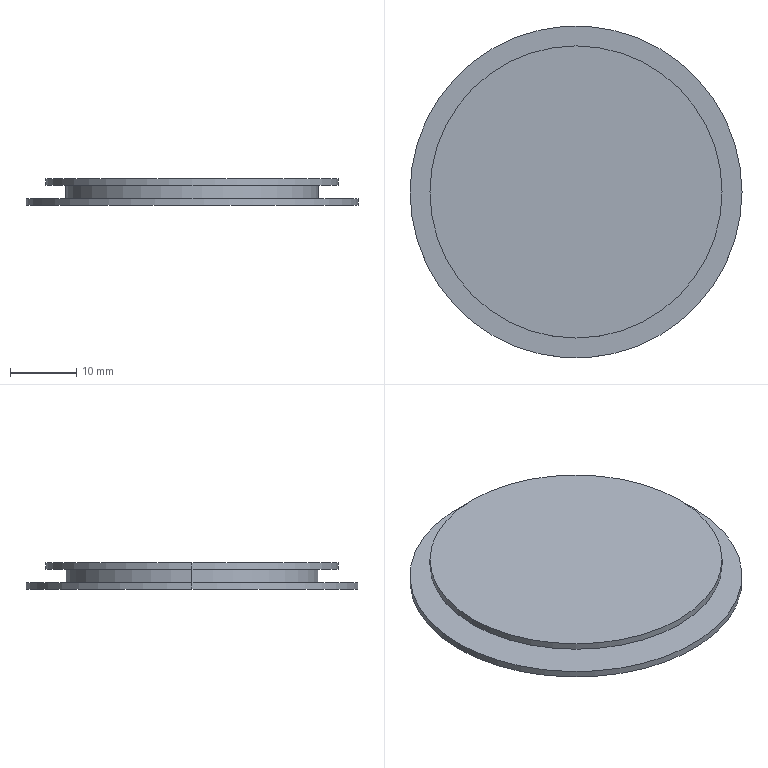Part | SolidWorks | features ICE 2, Extrusion 1 | 1 solid | 10 faces | box 50 x 50 x 4 mm | volume 5752 mm3 | cylinder 6 | plane 4 | commonest cylinder face diameters 38 x2 44 x2 50 x2
STEP:
#1=CARTESIAN_POINT('',(22.,0.,4.));
#2=VERTEX_POINT('',#1);
#3=CARTESIAN_POINT('',(-22.,0.,4.));
#4=VERTEX_POINT('',#3);
#5=CARTESIAN_POINT('',(0.,0.,4.));
#6=DIRECTION('',(0.,0.,1.));
#7=DIRECTION('',(1.,0.,0.));
#8=AXIS2_PLACEMENT_3D('',#5,#6,#7);
#9=CIRCLE('',#8,22.);
#10=EDGE_CURVE('',#2,#4,#9,.T.);
#11=ORIENTED_EDGE('',*,*,#10,.F.);
#12=CARTESIAN_POINT('',(22.,0.,3.));
#13=VERTEX_POINT('',#12);
#14=CARTESIAN_POINT('',(22.,0.,4.));
#15=DIRECTION('',(0.,0.,-1.));
#16=VECTOR('',#15,1000.);
#17=LINE('',#14,#16);
#18=EDGE_CURVE('',#2,#13,#17,.T.);
#19=ORIENTED_EDGE('',*,*,#18,.T.);
#20=CARTESIAN_POINT('',(-22.,0.,3.));
#21=VERTEX_POINT('',#20);
#22=CARTESIAN_POINT('',(0.,0.,3.));
#23=DIRECTION('',(0.,0.,1.));
#24=DIRECTION('',(1.,0.,0.));
#25=AXIS2_PLACEMENT_3D('',#22,#23,#24);
#26=CIRCLE('',#25,22.);
#27=EDGE_CURVE('',#13,#21,#26,.T.);
#28=ORIENTED_EDGE('',*,*,#27,.T.);
#29=CARTESIAN_POINT('',(-22.,0.,4.));
#30=DIRECTION('',(0.,0.,-1.));
#31=VECTOR('',#30,1000.);
#32=LINE('',#29,#31);
#33=EDGE_CURVE('',#4,#21,#32,.T.);
#34=ORIENTED_EDGE('',*,*,#33,.F.);
#35=EDGE_LOOP('',(#11,#19,#28,#34));
#36=FACE_OUTER_BOUND('',#35,.T.);
#37=CARTESIAN_POINT('',(0.,0.,4.));
#38=DIRECTION('',(0.,0.,-1.));
#39=DIRECTION('',(-1.,0.,0.));
#40=AXIS2_PLACEMENT_3D('',#37,#38,#39);
#41=CYLINDRICAL_SURFACE('',#40,22.);
#42=ADVANCED_FACE('',(#36),#41,.T.);
#43=CARTESIAN_POINT('',(19.,0.,3.));
#44=VERTEX_POINT('',#43);
#45=CARTESIAN_POINT('',(-19.,0.,3.));
#46=VERTEX_POINT('',#45);
#47=CARTESIAN_POINT('',(0.,0.,3.));
#48=DIRECTION('',(0.,0.,1.));
#49=DIRECTION('',(1.,0.,0.));
#50=AXIS2_PLACEMENT_3D('',#47,#48,#49);
#51=CIRCLE('',#50,19.);
#52=EDGE_CURVE('',#44,#46,#51,.T.);
#53=ORIENTED_EDGE('',*,*,#52,.F.);
#54=CARTESIAN_POINT('',(19.,0.,1.));
#55=VERTEX_POINT('',#54);
#56=CARTESIAN_POINT('',(19.,0.,3.));
#57=DIRECTION('',(0.,0.,-1.));
#58=VECTOR('',#57,1000.);
#59=LINE('',#56,#58);
#60=EDGE_CURVE('',#44,#55,#59,.T.);
#61=ORIENTED_EDGE('',*,*,#60,.T.);
#62=CARTESIAN_POINT('',(-19.,0.,1.));
#63=VERTEX_POINT('',#62);
#64=CARTESIAN_POINT('',(0.,0.,1.));
#65=DIRECTION('',(0.,0.,1.));
#66=DIRECTION('',(1.,0.,0.));
#67=AXIS2_PLACEMENT_3D('',#64,#65,#66);
#68=CIRCLE('',#67,19.);
#69=EDGE_CURVE('',#55,#63,#68,.T.);
#70=ORIENTED_EDGE('',*,*,#69,.T.);
#71=CARTESIAN_POINT('',(-19.,0.,3.));
#72=DIRECTION('',(0.,0.,-1.));
#73=VECTOR('',#72,1000.);
#74=LINE('',#71,#73);
#75=EDGE_CURVE('',#46,#63,#74,.T.);
#76=ORIENTED_EDGE('',*,*,#75,.F.);
#77=EDGE_LOOP('',(#53,#61,#70,#76));
#78=FACE_OUTER_BOUND('',#77,.T.);
#79=CARTESIAN_POINT('',(0.,0.,3.));
#80=DIRECTION('',(0.,0.,-1.));
#81=DIRECTION('',(-1.,0.,0.));
#82=AXIS2_PLACEMENT_3D('',#79,#80,#81);
#83=CYLINDRICAL_SURFACE('',#82,19.);
#84=ADVANCED_FACE('',(#78),#83,.T.);
#85=CARTESIAN_POINT('',(25.,0.,1.));
#86=VERTEX_POINT('',#85);
#87=CARTESIAN_POINT('',(-25.,0.,1.));
#88=VERTEX_POINT('',#87);
#89=CARTESIAN_POINT('',(0.,0.,1.));
#90=DIRECTION('',(0.,0.,1.));
#91=DIRECTION('',(1.,0.,0.));
#92=AXIS2_PLACEMENT_3D('',#89,#90,#91);
#93=CIRCLE('',#92,25.);
#94=EDGE_CURVE('',#86,#88,#93,.T.);
#95=ORIENTED_EDGE('',*,*,#94,.F.);
#96=CARTESIAN_POINT('',(25.,0.,0.));
#97=VERTEX_POINT('',#96);
#98=CARTESIAN_POINT('',(25.,0.,1.));
#99=DIRECTION('',(0.,0.,-1.));
#100=VECTOR('',#99,1000.);
#101=LINE('',#98,#100);
#102=EDGE_CURVE('',#86,#97,#101,.T.);
#103=ORIENTED_EDGE('',*,*,#102,.T.);
#104=CARTESIAN_POINT('',(-25.,0.,0.));
#105=VERTEX_POINT('',#104);
#106=CARTESIAN_POINT('',(0.,0.,0.));
#107=DIRECTION('',(0.,0.,1.));
#108=DIRECTION('',(1.,0.,0.));
#109=AXIS2_PLACEMENT_3D('',#106,#107,#108);
#110=CIRCLE('',#109,25.);
#111=EDGE_CURVE('',#97,#105,#110,.T.);
#112=ORIENTED_EDGE('',*,*,#111,.T.);
#113=CARTESIAN_POINT('',(-25.,0.,1.));
#114=DIRECTION('',(0.,0.,-1.));
#115=VECTOR('',#114,1000.);
#116=LINE('',#113,#115);
#117=EDGE_CURVE('',#88,#105,#116,.T.);
#118=ORIENTED_EDGE('',*,*,#117,.F.);
#119=EDGE_LOOP('',(#95,#103,#112,#118));
#120=FACE_OUTER_BOUND('',#119,.T.);
#121=CARTESIAN_POINT('',(0.,0.,1.));
#122=DIRECTION('',(0.,0.,-1.));
#123=DIRECTION('',(-1.,0.,0.));
#124=AXIS2_PLACEMENT_3D('',#121,#122,#123);
#125=CYLINDRICAL_SURFACE('',#124,25.);
#126=ADVANCED_FACE('',(#120),#125,.T.);
#127=ORIENTED_EDGE('',*,*,#102,.F.);
#128=CARTESIAN_POINT('',(0.,0.,1.));
#129=DIRECTION('',(0.,0.,1.));
#130=DIRECTION('',(1.,0.,0.));
#131=AXIS2_PLACEMENT_3D('',#128,#129,#130);
#132=CIRCLE('',#131,25.);
#133=EDGE_CURVE('',#88,#86,#132,.T.);
#134=ORIENTED_EDGE('',*,*,#133,.F.);
#135=ORIENTED_EDGE('',*,*,#117,.T.);
#136=CARTESIAN_POINT('',(0.,0.,0.));
#137=DIRECTION('',(0.,0.,1.));
#138=DIRECTION('',(1.,0.,0.));
#139=AXIS2_PLACEMENT_3D('',#136,#137,#138);
#140=CIRCLE('',#139,25.);
#141=EDGE_CURVE('',#105,#97,#140,.T.);
#142=ORIENTED_EDGE('',*,*,#141,.T.);
#143=EDGE_LOOP('',(#127,#134,#135,#142));
#144=FACE_OUTER_BOUND('',#143,.T.);
#145=CARTESIAN_POINT('',(0.,0.,1.));
#146=DIRECTION('',(0.,0.,-1.));
#147=DIRECTION('',(-1.,0.,0.));
#148=AXIS2_PLACEMENT_3D('',#145,#146,#147);
#149=CYLINDRICAL_SURFACE('',#148,25.);
#150=ADVANCED_FACE('',(#144),#149,.T.);
#151=CARTESIAN_POINT('',(0.,0.,1.));
#152=DIRECTION('',(0.,0.,1.));
#153=DIRECTION('',(1.,0.,0.));
#154=AXIS2_PLACEMENT_3D('',#151,#152,#153);
#155=CIRCLE('',#154,19.);
#156=EDGE_CURVE('',#63,#55,#155,.T.);
#157=ORIENTED_EDGE('',*,*,#156,.F.);
#158=ORIENTED_EDGE('',*,*,#69,.F.);
#159=EDGE_LOOP('',(#157,#158));
#160=FACE_BOUND('',#159,.T.);
#161=ORIENTED_EDGE('',*,*,#133,.T.);
#162=ORIENTED_EDGE('',*,*,#94,.T.);
#163=EDGE_LOOP('',(#161,#162));
#164=FACE_OUTER_BOUND('',#163,.T.);
#165=CARTESIAN_POINT('',(0.,0.,1.));
#166=DIRECTION('',(0.,0.,1.));
#167=DIRECTION('',(1.,0.,0.));
#168=AXIS2_PLACEMENT_3D('',#165,#166,#167);
#169=PLANE('',#168);
#170=ADVANCED_FACE('',(#160,#164),#169,.T.);
#171=ORIENTED_EDGE('',*,*,#141,.F.);
#172=ORIENTED_EDGE('',*,*,#111,.F.);
#173=EDGE_LOOP('',(#171,#172));
#174=FACE_OUTER_BOUND('',#173,.T.);
#175=CARTESIAN_POINT('',(0.,0.,0.));
#176=DIRECTION('',(0.,0.,1.));
#177=DIRECTION('',(1.,0.,0.));
#178=AXIS2_PLACEMENT_3D('',#175,#176,#177);
#179=PLANE('',#178);
#180=ADVANCED_FACE('',(#174),#179,.F.);
#181=ORIENTED_EDGE('',*,*,#60,.F.);
#182=CARTESIAN_POINT('',(0.,0.,3.));
#183=DIRECTION('',(0.,0.,1.));
#184=DIRECTION('',(1.,0.,0.));
#185=AXIS2_PLACEMENT_3D('',#182,#183,#184);
#186=CIRCLE('',#185,19.);
#187=EDGE_CURVE('',#46,#44,#186,.T.);
#188=ORIENTED_EDGE('',*,*,#187,.F.);
#189=ORIENTED_EDGE('',*,*,#75,.T.);
#190=ORIENTED_EDGE('',*,*,#156,.T.);
#191=EDGE_LOOP('',(#181,#188,#189,#190));
#192=FACE_OUTER_BOUND('',#191,.T.);
#193=CARTESIAN_POINT('',(0.,0.,3.));
#194=DIRECTION('',(0.,0.,-1.));
#195=DIRECTION('',(-1.,0.,0.));
#196=AXIS2_PLACEMENT_3D('',#193,#194,#195);
#197=CYLINDRICAL_SURFACE('',#196,19.);
#198=ADVANCED_FACE('',(#192),#197,.T.);
#199=ORIENTED_EDGE('',*,*,#18,.F.);
#200=CARTESIAN_POINT('',(0.,0.,4.));
#201=DIRECTION('',(0.,0.,1.));
#202=DIRECTION('',(1.,0.,0.));
#203=AXIS2_PLACEMENT_3D('',#200,#201,#202);
#204=CIRCLE('',#203,22.);
#205=EDGE_CURVE('',#4,#2,#204,.T.);
#206=ORIENTED_EDGE('',*,*,#205,.F.);
#207=ORIENTED_EDGE('',*,*,#33,.T.);
#208=CARTESIAN_POINT('',(0.,0.,3.));
#209=DIRECTION('',(0.,0.,1.));
#210=DIRECTION('',(1.,0.,0.));
#211=AXIS2_PLACEMENT_3D('',#208,#209,#210);
#212=CIRCLE('',#211,22.);
#213=EDGE_CURVE('',#21,#13,#212,.T.);
#214=ORIENTED_EDGE('',*,*,#213,.T.);
#215=EDGE_LOOP('',(#199,#206,#207,#214));
#216=FACE_OUTER_BOUND('',#215,.T.);
#217=CARTESIAN_POINT('',(0.,0.,4.));
#218=DIRECTION('',(0.,0.,-1.));
#219=DIRECTION('',(-1.,0.,0.));
#220=AXIS2_PLACEMENT_3D('',#217,#218,#219);
#221=CYLINDRICAL_SURFACE('',#220,22.);
#222=ADVANCED_FACE('',(#216),#221,.T.);
#223=ORIENTED_EDGE('',*,*,#205,.T.);
#224=ORIENTED_EDGE('',*,*,#10,.T.);
#225=EDGE_LOOP('',(#223,#224));
#226=FACE_OUTER_BOUND('',#225,.T.);
#227=CARTESIAN_POINT('',(0.,0.,4.));
#228=DIRECTION('',(0.,0.,1.));
#229=DIRECTION('',(1.,0.,0.));
#230=AXIS2_PLACEMENT_3D('',#227,#228,#229);
#231=PLANE('',#230);
#232=ADVANCED_FACE('',(#226),#231,.T.);
#233=ORIENTED_EDGE('',*,*,#187,.T.);
#234=ORIENTED_EDGE('',*,*,#52,.T.);
#235=EDGE_LOOP('',(#233,#234));
#236=FACE_BOUND('',#235,.T.);
#237=ORIENTED_EDGE('',*,*,#213,.F.);
#238=ORIENTED_EDGE('',*,*,#27,.F.);
#239=EDGE_LOOP('',(#237,#238));
#240=FACE_OUTER_BOUND('',#239,.T.);
#241=CARTESIAN_POINT('',(0.,0.,3.));
#242=DIRECTION('',(0.,0.,1.));
#243=DIRECTION('',(1.,0.,0.));
#244=AXIS2_PLACEMENT_3D('',#241,#242,#243);
#245=PLANE('',#244);
#246=ADVANCED_FACE('',(#236,#240),#245,.F.);
#247=CLOSED_SHELL('',(#42,#84,#126,#150,#170,#180,#198,#222,#232,#246));
#248=MANIFOLD_SOLID_BREP('',#247);
#249=CARTESIAN_POINT('',(0.,0.,0.));
#250=DIRECTION('',(0.,0.,1.));
#251=DIRECTION('',(1.,0.,0.));
#252=AXIS2_PLACEMENT_3D('',#249,#250,#251);
#253=(LENGTH_UNIT()NAMED_UNIT(*)SI_UNIT(.MILLI.,.METRE.));
#254=UNCERTAINTY_MEASURE_WITH_UNIT(LENGTH_MEASURE(0.00001),#253,'','');
#255=(NAMED_UNIT(*)PLANE_ANGLE_UNIT()SI_UNIT($,.RADIAN.));
#256=(NAMED_UNIT(*)SI_UNIT($,.STERADIAN.)SOLID_ANGLE_UNIT());
#257=(GEOMETRIC_REPRESENTATION_CONTEXT(3)GLOBAL_UNCERTAINTY_ASSIGNED_CONTEXT((#254))GLOBAL_UNIT_ASSIGNED_CONTEXT((#253,#255,#256))REPRESENTATION_CONTEXT('',''));
#258=ADVANCED_BREP_SHAPE_REPRESENTATION('',(#248,#252),#257);